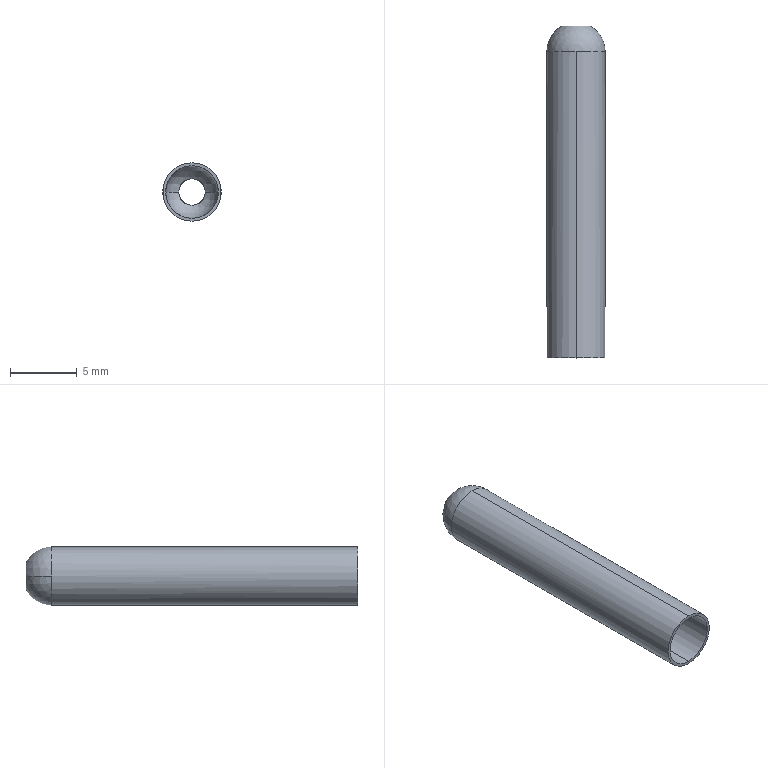Part | SolidWorks | features Revolution 1 | 1 solid | 12 faces | box 4.36 x 24.8 x 4.36 mm | volume 67.655 mm3 | cylinder 6 | sphere 4 | plane 2 | commonest cylinder face diameters 1.989 x2 3.94 x2 4.36 x2
STEP:
#1=CARTESIAN_POINT('',(0.,22.89,1.97));
#2=VERTEX_POINT('',#1);
#3=CARTESIAN_POINT('',(-1.97,22.89,0.));
#4=VERTEX_POINT('',#3);
#5=CARTESIAN_POINT('',(0.,22.89,0.));
#6=DIRECTION('',(0.,-1.,0.));
#7=DIRECTION('',(0.,0.,-1.));
#8=AXIS2_PLACEMENT_3D('',#5,#6,#7);
#9=CIRCLE('',#8,1.97);
#10=EDGE_CURVE('',#2,#4,#9,.T.);
#11=ORIENTED_EDGE('',*,*,#10,.F.);
#12=CARTESIAN_POINT('',(0.,0.,1.97));
#13=VERTEX_POINT('',#12);
#14=CARTESIAN_POINT('',(0.,0.,1.97));
#15=DIRECTION('',(0.,-1.,0.));
#16=VECTOR('',#15,1000.);
#17=LINE('',#14,#16);
#18=EDGE_CURVE('',#2,#13,#17,.T.);
#19=ORIENTED_EDGE('',*,*,#18,.T.);
#20=CARTESIAN_POINT('',(0.,0.,-1.97));
#21=VERTEX_POINT('',#20);
#22=CARTESIAN_POINT('',(0.,0.,0.));
#23=DIRECTION('',(0.,-1.,0.));
#24=DIRECTION('',(0.,0.,-1.));
#25=AXIS2_PLACEMENT_3D('',#22,#23,#24);
#26=CIRCLE('',#25,1.97);
#27=EDGE_CURVE('',#13,#21,#26,.T.);
#28=ORIENTED_EDGE('',*,*,#27,.T.);
#29=CARTESIAN_POINT('',(0.,22.89,-1.97));
#30=VERTEX_POINT('',#29);
#31=CARTESIAN_POINT('',(0.,0.,-1.97));
#32=DIRECTION('',(0.,-1.,0.));
#33=VECTOR('',#32,1000.);
#34=LINE('',#31,#33);
#35=EDGE_CURVE('',#30,#21,#34,.T.);
#36=ORIENTED_EDGE('',*,*,#35,.F.);
#37=CARTESIAN_POINT('',(0.,22.89,0.));
#38=DIRECTION('',(0.,-1.,0.));
#39=DIRECTION('',(0.,0.,-1.));
#40=AXIS2_PLACEMENT_3D('',#37,#38,#39);
#41=CIRCLE('',#40,1.97);
#42=EDGE_CURVE('',#4,#30,#41,.T.);
#43=ORIENTED_EDGE('',*,*,#42,.F.);
#44=EDGE_LOOP('',(#11,#19,#28,#36,#43));
#45=FACE_OUTER_BOUND('',#44,.T.);
#46=CARTESIAN_POINT('',(0.,0.,0.));
#47=DIRECTION('',(0.,-1.,0.));
#48=DIRECTION('',(0.,0.,-1.));
#49=AXIS2_PLACEMENT_3D('',#46,#47,#48);
#50=CYLINDRICAL_SURFACE('',#49,1.97);
#51=ADVANCED_FACE('',(#45),#50,.F.);
#52=CARTESIAN_POINT('',(0.9946,24.59,0.));
#53=VERTEX_POINT('',#52);
#54=CARTESIAN_POINT('',(0.,24.59,0.9946));
#55=VERTEX_POINT('',#54);
#56=CARTESIAN_POINT('',(0.,24.59,0.));
#57=DIRECTION('',(0.,-1.,0.));
#58=DIRECTION('',(0.,0.,-1.));
#59=AXIS2_PLACEMENT_3D('',#56,#57,#58);
#60=CIRCLE('',#59,0.9946);
#61=EDGE_CURVE('',#53,#55,#60,.T.);
#62=ORIENTED_EDGE('',*,*,#61,.F.);
#63=CARTESIAN_POINT('',(1.97,22.89,0.));
#64=VERTEX_POINT('',#63);
#65=CARTESIAN_POINT('',(0.,22.89,0.));
#66=DIRECTION('',(0.,0.,-1.));
#67=DIRECTION('',(-1.,0.,0.));
#68=AXIS2_PLACEMENT_3D('',#65,#66,#67);
#69=CIRCLE('',#68,1.97);
#70=EDGE_CURVE('',#53,#64,#69,.T.);
#71=ORIENTED_EDGE('',*,*,#70,.T.);
#72=CARTESIAN_POINT('',(0.,22.89,0.));
#73=DIRECTION('',(0.,-1.,0.));
#74=DIRECTION('',(0.,0.,-1.));
#75=AXIS2_PLACEMENT_3D('',#72,#73,#74);
#76=CIRCLE('',#75,1.97);
#77=EDGE_CURVE('',#64,#2,#76,.T.);
#78=ORIENTED_EDGE('',*,*,#77,.T.);
#79=ORIENTED_EDGE('',*,*,#10,.T.);
#80=CARTESIAN_POINT('',(-0.9946,24.59,0.));
#81=VERTEX_POINT('',#80);
#82=CARTESIAN_POINT('',(0.,22.89,0.));
#83=DIRECTION('',(0.,0.,1.));
#84=DIRECTION('',(1.,0.,0.));
#85=AXIS2_PLACEMENT_3D('',#82,#83,#84);
#86=CIRCLE('',#85,1.97);
#87=EDGE_CURVE('',#81,#4,#86,.T.);
#88=ORIENTED_EDGE('',*,*,#87,.F.);
#89=CARTESIAN_POINT('',(0.,24.59,0.));
#90=DIRECTION('',(0.,-1.,0.));
#91=DIRECTION('',(0.,0.,-1.));
#92=AXIS2_PLACEMENT_3D('',#89,#90,#91);
#93=CIRCLE('',#92,0.9946);
#94=EDGE_CURVE('',#55,#81,#93,.T.);
#95=ORIENTED_EDGE('',*,*,#94,.F.);
#96=EDGE_LOOP('',(#62,#71,#78,#79,#88,#95));
#97=FACE_OUTER_BOUND('',#96,.T.);
#98=CARTESIAN_POINT('',(0.,22.89,0.));
#99=DIRECTION('',(0.,0.,-1.));
#100=DIRECTION('',(-1.,0.,0.));
#101=AXIS2_PLACEMENT_3D('',#98,#99,#100);
#102=SPHERICAL_SURFACE('',#101,1.97);
#103=ADVANCED_FACE('',(#97),#102,.F.);
#104=CARTESIAN_POINT('',(0.,24.8,0.9946));
#105=VERTEX_POINT('',#104);
#106=CARTESIAN_POINT('',(0.,24.8,-0.9946));
#107=VERTEX_POINT('',#106);
#108=CARTESIAN_POINT('',(0.,24.8,0.));
#109=DIRECTION('',(0.,-1.,0.));
#110=DIRECTION('',(0.,0.,-1.));
#111=AXIS2_PLACEMENT_3D('',#108,#109,#110);
#112=CIRCLE('',#111,0.9946);
#113=EDGE_CURVE('',#105,#107,#112,.T.);
#114=ORIENTED_EDGE('',*,*,#113,.F.);
#115=CARTESIAN_POINT('',(0.,0.,0.9946));
#116=DIRECTION('',(0.,-1.,0.));
#117=VECTOR('',#116,1000.);
#118=LINE('',#115,#117);
#119=EDGE_CURVE('',#105,#55,#118,.T.);
#120=ORIENTED_EDGE('',*,*,#119,.T.);
#121=ORIENTED_EDGE('',*,*,#94,.T.);
#122=CARTESIAN_POINT('',(0.,24.59,-0.9946));
#123=VERTEX_POINT('',#122);
#124=CARTESIAN_POINT('',(0.,24.59,0.));
#125=DIRECTION('',(0.,-1.,0.));
#126=DIRECTION('',(0.,0.,-1.));
#127=AXIS2_PLACEMENT_3D('',#124,#125,#126);
#128=CIRCLE('',#127,0.9946);
#129=EDGE_CURVE('',#81,#123,#128,.T.);
#130=ORIENTED_EDGE('',*,*,#129,.T.);
#131=CARTESIAN_POINT('',(0.,0.,-0.9946));
#132=DIRECTION('',(0.,-1.,0.));
#133=VECTOR('',#132,1000.);
#134=LINE('',#131,#133);
#135=EDGE_CURVE('',#107,#123,#134,.T.);
#136=ORIENTED_EDGE('',*,*,#135,.F.);
#137=EDGE_LOOP('',(#114,#120,#121,#130,#136));
#138=FACE_OUTER_BOUND('',#137,.T.);
#139=CARTESIAN_POINT('',(0.,0.,0.));
#140=DIRECTION('',(0.,-1.,0.));
#141=DIRECTION('',(0.,0.,-1.));
#142=AXIS2_PLACEMENT_3D('',#139,#140,#141);
#143=CYLINDRICAL_SURFACE('',#142,0.9946);
#144=ADVANCED_FACE('',(#138),#143,.F.);
#145=CARTESIAN_POINT('',(-1.05,24.8,0.));
#146=VERTEX_POINT('',#145);
#147=CARTESIAN_POINT('',(1.05,24.8,0.));
#148=VERTEX_POINT('',#147);
#149=CARTESIAN_POINT('',(0.,24.8,0.));
#150=DIRECTION('',(0.,-1.,0.));
#151=DIRECTION('',(0.,0.,-1.));
#152=AXIS2_PLACEMENT_3D('',#149,#150,#151);
#153=CIRCLE('',#152,1.05);
#154=EDGE_CURVE('',#146,#148,#153,.T.);
#155=ORIENTED_EDGE('',*,*,#154,.T.);
#156=CARTESIAN_POINT('',(2.18,22.89,0.));
#157=VERTEX_POINT('',#156);
#158=CARTESIAN_POINT('',(0.,22.89,0.));
#159=DIRECTION('',(0.,0.,-1.));
#160=DIRECTION('',(-1.,0.,0.));
#161=AXIS2_PLACEMENT_3D('',#158,#159,#160);
#162=CIRCLE('',#161,2.18);
#163=EDGE_CURVE('',#148,#157,#162,.T.);
#164=ORIENTED_EDGE('',*,*,#163,.T.);
#165=CARTESIAN_POINT('',(0.,22.89,-2.18));
#166=VERTEX_POINT('',#165);
#167=CARTESIAN_POINT('',(0.,22.89,0.));
#168=DIRECTION('',(0.,-1.,0.));
#169=DIRECTION('',(0.,0.,-1.));
#170=AXIS2_PLACEMENT_3D('',#167,#168,#169);
#171=CIRCLE('',#170,2.18);
#172=EDGE_CURVE('',#166,#157,#171,.T.);
#173=ORIENTED_EDGE('',*,*,#172,.F.);
#174=CARTESIAN_POINT('',(-2.18,22.89,0.));
#175=VERTEX_POINT('',#174);
#176=CARTESIAN_POINT('',(0.,22.89,0.));
#177=DIRECTION('',(0.,-1.,0.));
#178=DIRECTION('',(0.,0.,-1.));
#179=AXIS2_PLACEMENT_3D('',#176,#177,#178);
#180=CIRCLE('',#179,2.18);
#181=EDGE_CURVE('',#175,#166,#180,.T.);
#182=ORIENTED_EDGE('',*,*,#181,.F.);
#183=CARTESIAN_POINT('',(0.,22.89,0.));
#184=DIRECTION('',(0.,0.,1.));
#185=DIRECTION('',(1.,0.,0.));
#186=AXIS2_PLACEMENT_3D('',#183,#184,#185);
#187=CIRCLE('',#186,2.18);
#188=EDGE_CURVE('',#146,#175,#187,.T.);
#189=ORIENTED_EDGE('',*,*,#188,.F.);
#190=EDGE_LOOP('',(#155,#164,#173,#182,#189));
#191=FACE_OUTER_BOUND('',#190,.T.);
#192=CARTESIAN_POINT('',(0.,22.89,0.));
#193=DIRECTION('',(0.,0.,-1.));
#194=DIRECTION('',(-1.,0.,0.));
#195=AXIS2_PLACEMENT_3D('',#192,#193,#194);
#196=SPHERICAL_SURFACE('',#195,2.18);
#197=ADVANCED_FACE('',(#191),#196,.T.);
#198=ORIENTED_EDGE('',*,*,#172,.T.);
#199=CARTESIAN_POINT('',(0.,22.89,2.18));
#200=VERTEX_POINT('',#199);
#201=CARTESIAN_POINT('',(0.,22.89,0.));
#202=DIRECTION('',(0.,-1.,0.));
#203=DIRECTION('',(0.,0.,-1.));
#204=AXIS2_PLACEMENT_3D('',#201,#202,#203);
#205=CIRCLE('',#204,2.18);
#206=EDGE_CURVE('',#157,#200,#205,.T.);
#207=ORIENTED_EDGE('',*,*,#206,.T.);
#208=CARTESIAN_POINT('',(0.,0.,2.18));
#209=VERTEX_POINT('',#208);
#210=CARTESIAN_POINT('',(0.,0.,2.18));
#211=DIRECTION('',(0.,-1.,0.));
#212=VECTOR('',#211,1000.);
#213=LINE('',#210,#212);
#214=EDGE_CURVE('',#200,#209,#213,.T.);
#215=ORIENTED_EDGE('',*,*,#214,.T.);
#216=CARTESIAN_POINT('',(0.,0.,-2.18));
#217=VERTEX_POINT('',#216);
#218=CARTESIAN_POINT('',(0.,0.,0.));
#219=DIRECTION('',(0.,-1.,0.));
#220=DIRECTION('',(0.,0.,-1.));
#221=AXIS2_PLACEMENT_3D('',#218,#219,#220);
#222=CIRCLE('',#221,2.18);
#223=EDGE_CURVE('',#217,#209,#222,.T.);
#224=ORIENTED_EDGE('',*,*,#223,.F.);
#225=CARTESIAN_POINT('',(0.,0.,-2.18));
#226=DIRECTION('',(0.,-1.,0.));
#227=VECTOR('',#226,1000.);
#228=LINE('',#225,#227);
#229=EDGE_CURVE('',#166,#217,#228,.T.);
#230=ORIENTED_EDGE('',*,*,#229,.F.);
#231=EDGE_LOOP('',(#198,#207,#215,#224,#230));
#232=FACE_OUTER_BOUND('',#231,.T.);
#233=CARTESIAN_POINT('',(0.,0.,0.));
#234=DIRECTION('',(0.,-1.,0.));
#235=DIRECTION('',(0.,0.,-1.));
#236=AXIS2_PLACEMENT_3D('',#233,#234,#235);
#237=CYLINDRICAL_SURFACE('',#236,2.18);
#238=ADVANCED_FACE('',(#232),#237,.T.);
#239=CARTESIAN_POINT('',(0.,0.,0.));
#240=DIRECTION('',(0.,-1.,0.));
#241=DIRECTION('',(0.,0.,-1.));
#242=AXIS2_PLACEMENT_3D('',#239,#240,#241);
#243=CIRCLE('',#242,1.97);
#244=EDGE_CURVE('',#21,#13,#243,.T.);
#245=ORIENTED_EDGE('',*,*,#244,.F.);
#246=ORIENTED_EDGE('',*,*,#27,.F.);
#247=EDGE_LOOP('',(#245,#246));
#248=FACE_BOUND('',#247,.T.);
#249=ORIENTED_EDGE('',*,*,#223,.T.);
#250=CARTESIAN_POINT('',(0.,0.,0.));
#251=DIRECTION('',(0.,-1.,0.));
#252=DIRECTION('',(0.,0.,-1.));
#253=AXIS2_PLACEMENT_3D('',#250,#251,#252);
#254=CIRCLE('',#253,2.18);
#255=EDGE_CURVE('',#209,#217,#254,.T.);
#256=ORIENTED_EDGE('',*,*,#255,.T.);
#257=EDGE_LOOP('',(#249,#256));
#258=FACE_OUTER_BOUND('',#257,.T.);
#259=CARTESIAN_POINT('',(-2.18,0.,0.));
#260=DIRECTION('',(0.,1.,0.));
#261=DIRECTION('',(0.,0.,1.));
#262=AXIS2_PLACEMENT_3D('',#259,#260,#261);
#263=PLANE('',#262);
#264=ADVANCED_FACE('',(#248,#258),#263,.F.);
#265=ORIENTED_EDGE('',*,*,#214,.F.);
#266=CARTESIAN_POINT('',(0.,22.89,0.));
#267=DIRECTION('',(0.,-1.,0.));
#268=DIRECTION('',(0.,0.,-1.));
#269=AXIS2_PLACEMENT_3D('',#266,#267,#268);
#270=CIRCLE('',#269,2.18);
#271=EDGE_CURVE('',#200,#175,#270,.T.);
#272=ORIENTED_EDGE('',*,*,#271,.T.);
#273=ORIENTED_EDGE('',*,*,#181,.T.);
#274=ORIENTED_EDGE('',*,*,#229,.T.);
#275=ORIENTED_EDGE('',*,*,#255,.F.);
#276=EDGE_LOOP('',(#265,#272,#273,#274,#275));
#277=FACE_OUTER_BOUND('',#276,.T.);
#278=CARTESIAN_POINT('',(0.,0.,0.));
#279=DIRECTION('',(0.,-1.,0.));
#280=DIRECTION('',(0.,0.,-1.));
#281=AXIS2_PLACEMENT_3D('',#278,#279,#280);
#282=CYLINDRICAL_SURFACE('',#281,2.18);
#283=ADVANCED_FACE('',(#277),#282,.T.);
#284=ORIENTED_EDGE('',*,*,#163,.F.);
#285=CARTESIAN_POINT('',(0.,24.8,0.));
#286=DIRECTION('',(0.,-1.,0.));
#287=DIRECTION('',(0.,0.,-1.));
#288=AXIS2_PLACEMENT_3D('',#285,#286,#287);
#289=CIRCLE('',#288,1.05);
#290=EDGE_CURVE('',#148,#146,#289,.T.);
#291=ORIENTED_EDGE('',*,*,#290,.T.);
#292=ORIENTED_EDGE('',*,*,#188,.T.);
#293=ORIENTED_EDGE('',*,*,#271,.F.);
#294=ORIENTED_EDGE('',*,*,#206,.F.);
#295=EDGE_LOOP('',(#284,#291,#292,#293,#294));
#296=FACE_OUTER_BOUND('',#295,.T.);
#297=CARTESIAN_POINT('',(0.,22.89,0.));
#298=DIRECTION('',(0.,0.,-1.));
#299=DIRECTION('',(-1.,0.,0.));
#300=AXIS2_PLACEMENT_3D('',#297,#298,#299);
#301=SPHERICAL_SURFACE('',#300,2.18);
#302=ADVANCED_FACE('',(#296),#301,.T.);
#303=ORIENTED_EDGE('',*,*,#154,.F.);
#304=ORIENTED_EDGE('',*,*,#290,.F.);
#305=EDGE_LOOP('',(#303,#304));
#306=FACE_OUTER_BOUND('',#305,.T.);
#307=CARTESIAN_POINT('',(0.,24.8,0.));
#308=DIRECTION('',(0.,-1.,0.));
#309=DIRECTION('',(0.,0.,-1.));
#310=AXIS2_PLACEMENT_3D('',#307,#308,#309);
#311=CIRCLE('',#310,0.9946);
#312=EDGE_CURVE('',#107,#105,#311,.T.);
#313=ORIENTED_EDGE('',*,*,#312,.T.);
#314=ORIENTED_EDGE('',*,*,#113,.T.);
#315=EDGE_LOOP('',(#313,#314));
#316=FACE_BOUND('',#315,.T.);
#317=CARTESIAN_POINT('',(-1.05,24.8,0.));
#318=DIRECTION('',(0.,-1.,0.));
#319=DIRECTION('',(0.,0.,-1.));
#320=AXIS2_PLACEMENT_3D('',#317,#318,#319);
#321=PLANE('',#320);
#322=ADVANCED_FACE('',(#306,#316),#321,.F.);
#323=ORIENTED_EDGE('',*,*,#119,.F.);
#324=ORIENTED_EDGE('',*,*,#312,.F.);
#325=ORIENTED_EDGE('',*,*,#135,.T.);
#326=CARTESIAN_POINT('',(0.,24.59,0.));
#327=DIRECTION('',(0.,-1.,0.));
#328=DIRECTION('',(0.,0.,-1.));
#329=AXIS2_PLACEMENT_3D('',#326,#327,#328);
#330=CIRCLE('',#329,0.9946);
#331=EDGE_CURVE('',#123,#53,#330,.T.);
#332=ORIENTED_EDGE('',*,*,#331,.T.);
#333=ORIENTED_EDGE('',*,*,#61,.T.);
#334=EDGE_LOOP('',(#323,#324,#325,#332,#333));
#335=FACE_OUTER_BOUND('',#334,.T.);
#336=CARTESIAN_POINT('',(0.,0.,0.));
#337=DIRECTION('',(0.,-1.,0.));
#338=DIRECTION('',(0.,0.,-1.));
#339=AXIS2_PLACEMENT_3D('',#336,#337,#338);
#340=CYLINDRICAL_SURFACE('',#339,0.9946);
#341=ADVANCED_FACE('',(#335),#340,.F.);
#342=ORIENTED_EDGE('',*,*,#70,.F.);
#343=ORIENTED_EDGE('',*,*,#331,.F.);
#344=ORIENTED_EDGE('',*,*,#129,.F.);
#345=ORIENTED_EDGE('',*,*,#87,.T.);
#346=ORIENTED_EDGE('',*,*,#42,.T.);
#347=CARTESIAN_POINT('',(0.,22.89,0.));
#348=DIRECTION('',(0.,-1.,0.));
#349=DIRECTION('',(0.,0.,-1.));
#350=AXIS2_PLACEMENT_3D('',#347,#348,#349);
#351=CIRCLE('',#350,1.97);
#352=EDGE_CURVE('',#30,#64,#351,.T.);
#353=ORIENTED_EDGE('',*,*,#352,.T.);
#354=EDGE_LOOP('',(#342,#343,#344,#345,#346,#353));
#355=FACE_OUTER_BOUND('',#354,.T.);
#356=CARTESIAN_POINT('',(0.,22.89,0.));
#357=DIRECTION('',(0.,0.,-1.));
#358=DIRECTION('',(-1.,0.,0.));
#359=AXIS2_PLACEMENT_3D('',#356,#357,#358);
#360=SPHERICAL_SURFACE('',#359,1.97);
#361=ADVANCED_FACE('',(#355),#360,.F.);
#362=ORIENTED_EDGE('',*,*,#18,.F.);
#363=ORIENTED_EDGE('',*,*,#77,.F.);
#364=ORIENTED_EDGE('',*,*,#352,.F.);
#365=ORIENTED_EDGE('',*,*,#35,.T.);
#366=ORIENTED_EDGE('',*,*,#244,.T.);
#367=EDGE_LOOP('',(#362,#363,#364,#365,#366));
#368=FACE_OUTER_BOUND('',#367,.T.);
#369=CARTESIAN_POINT('',(0.,0.,0.));
#370=DIRECTION('',(0.,-1.,0.));
#371=DIRECTION('',(0.,0.,-1.));
#372=AXIS2_PLACEMENT_3D('',#369,#370,#371);
#373=CYLINDRICAL_SURFACE('',#372,1.97);
#374=ADVANCED_FACE('',(#368),#373,.F.);
#375=CLOSED_SHELL('',(#51,#103,#144,#197,#238,#264,#283,#302,#322,#341,#361,#374));
#376=MANIFOLD_SOLID_BREP('',#375);
#377=CARTESIAN_POINT('',(0.,0.,0.));
#378=DIRECTION('',(0.,0.,1.));
#379=DIRECTION('',(1.,0.,0.));
#380=AXIS2_PLACEMENT_3D('',#377,#378,#379);
#381=(LENGTH_UNIT()NAMED_UNIT(*)SI_UNIT(.MILLI.,.METRE.));
#382=UNCERTAINTY_MEASURE_WITH_UNIT(LENGTH_MEASURE(0.00001),#381,'','');
#383=(NAMED_UNIT(*)PLANE_ANGLE_UNIT()SI_UNIT($,.RADIAN.));
#384=(NAMED_UNIT(*)SI_UNIT($,.STERADIAN.)SOLID_ANGLE_UNIT());
#385=(GEOMETRIC_REPRESENTATION_CONTEXT(3)GLOBAL_UNCERTAINTY_ASSIGNED_CONTEXT((#382))GLOBAL_UNIT_ASSIGNED_CONTEXT((#381,#383,#384))REPRESENTATION_CONTEXT('',''));
#386=ADVANCED_BREP_SHAPE_REPRESENTATION('',(#376,#380),#385);